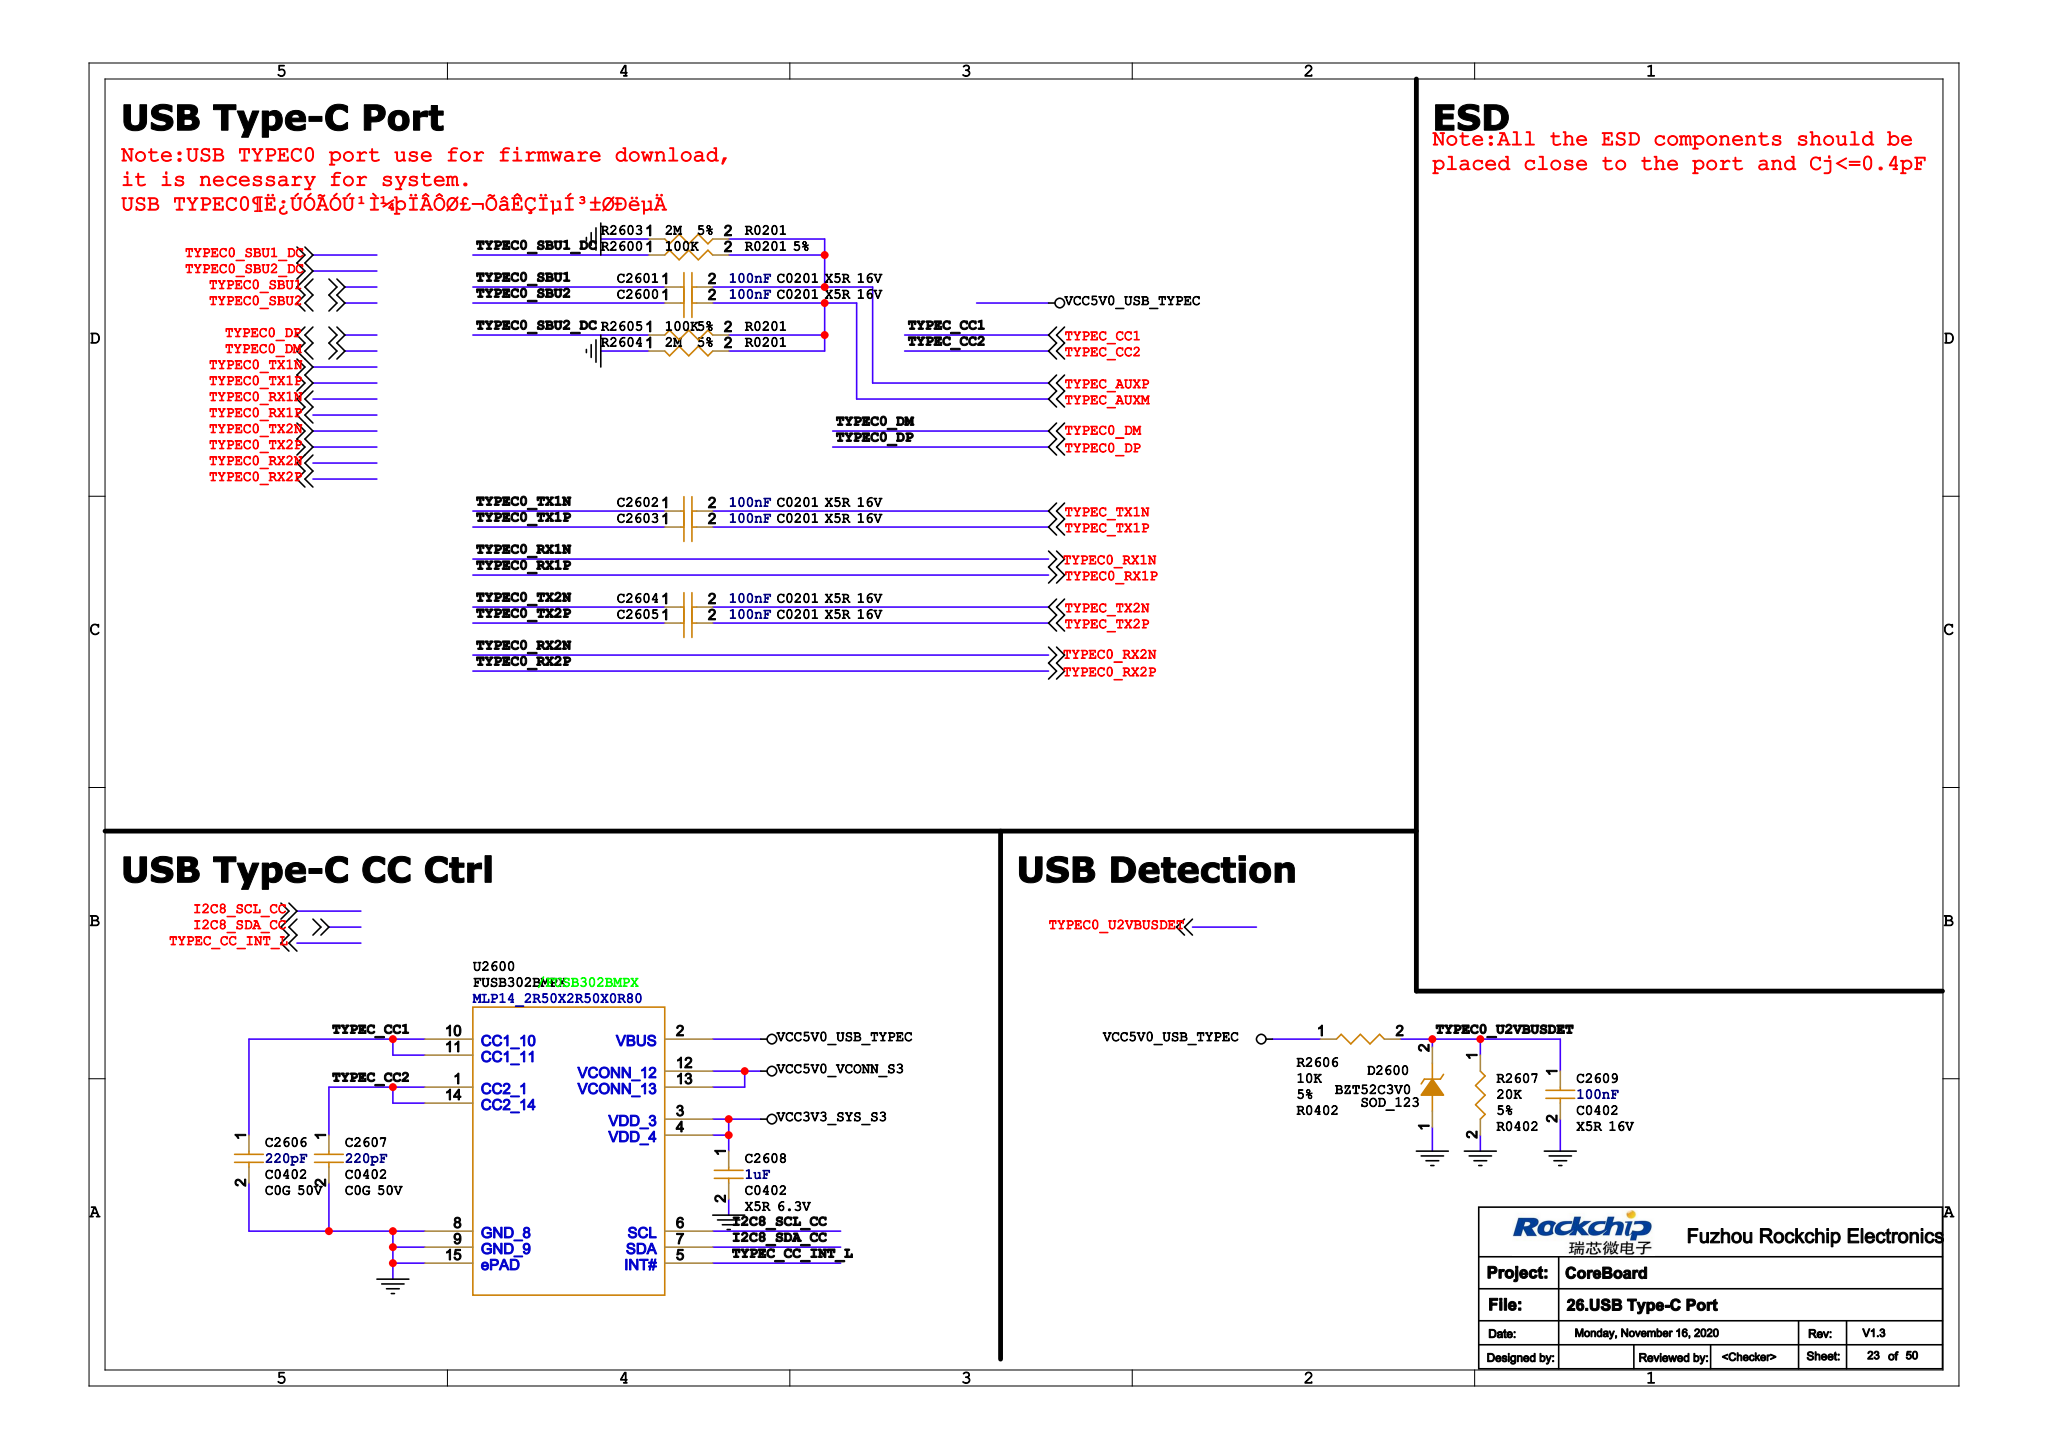Circuit board | Cadence Allegro | 749 parts | 717 nets | one sheet of the schematic
Parts on this sheet (reference | value | footprint):
C2606 | 220pF | C0402
C2607 | 220pF | C0402
C2608 | 1uF | C0402
C2609 | 100nF | C0402
D2600 | BZT52C3V0 | SOD_123
R2606 | 10K | R0402
R2607 | 20K | R0402
U2600 | FUSB302BMPX | MLP14_2R50X2R50X0R80
Nets of these parts (net: part-pin ...):
GND: C2606-2 C2607-2 C2608-2 C2609-2 D2600-1 R2607-2 U2600-8 U2600-9 U2600-15
TYPEC_CC1: C2606-1 U2600-10 U2600-11
TYPEC_CC2: C2607-1 U2600-1 U2600-14
TYPEC0_U2VBUSDET: C2609-1 D2600-2 R2606-2 R2607-1
VCC5V0_USB_TYPEC: R2606-1 U2600-2
TYPEC_CC_INT_L: U2600-5
I2C8_SCL_CC: U2600-6
I2C8_SDA_CC: U2600-7
VCC5V0_VCONN_S3: U2600-12 U2600-13
VCC3V3_SYS_S3: C2608-1 U2600-3 U2600-4